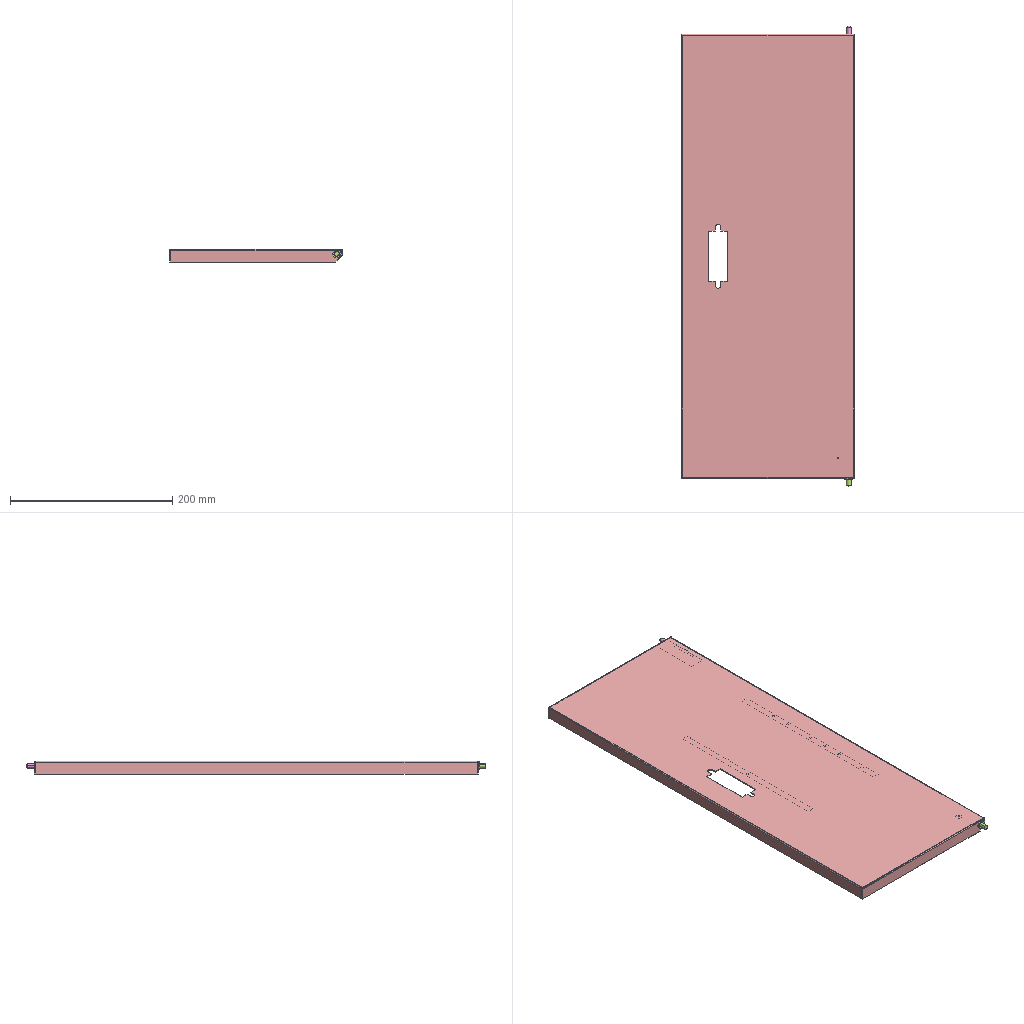Assembly | SolidWorks | 8 different items | 8 placed | box 213 x 566 x 17 mm
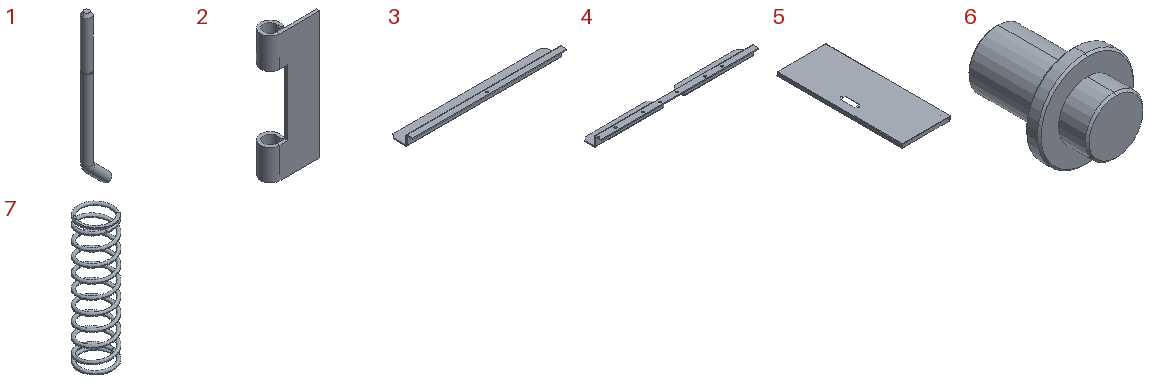Parts list (item | name | quantity | size | volume | features):
1 | - | x1 | 16.636 x 5.506 x 95.612 mm | 2325 mm3 | features Chamfer 2, ICE 2, Sweep 1
2 | - | x1 | 24 x 9.5 x 62 mm | 2570 mm3 | features FlatPattern 1, ICE 1, SMBaseFlange 1, SheetMetal 1
3 | - | x1 | 220 x 33.5 x 15 mm | 15208 mm3 | features EdgeFlange 2, ICE 2, Chamfer 1, FlatPattern 1, SMBaseFlange 1, SheetMetal 1
4 | - | x1 | 230 x 28.5 x 15 mm | 12722 mm3 | features LPattern 4, ICE 3, EdgeFlange 2, Chamfer 1, FlatPattern 1, SMBaseFlange 1, SheetMetal 1
5 | - | x1 | 213 x 547 x 16 mm | 163711 mm3 | features EdgeFlange 4, FlatPattern 1, ICE 1, SMBaseFlange 1, SheetMetal 1
6 | - | x1 | 10 x 12.5 x 10 mm | 426.85 mm3 | features ICE 2, Chamfer 1, Extrusion 1
7 | - | x1 | 8.799 x 8.797 x 32 mm | 125.702 mm3 | features BaseBody 1
8 | headless studs for stud welding gb | x1 | - | - | -
Mates (type | each side: item.copy, entity, surface, feature):
Coincident | 5.1 face plane Base-Flange1 | 2.1 face plane Base-Flange1
Coincident | 5.1 face plane Edge-Flange1 | 2.1 face plane Base-Bend1
DistanceDim | 2.1 face plane Base-Flange1 | 5.1 face plane Edge-Flange3
Concentric | 5.1 face cylinder Cut-Extrude1 | 6.1 face cylinder Boss-Extrude3
DistanceDim | 1.1 face plane Boss-Extrude2 | 5.1 face plane Edge-Flange1
Concentric | 2.1 face cylinder Base-Bend1 | 1.1 face cylinder Boss-Extrude2
Coincident | 2.1 face plane Cut-Extrude1 | 7.1 face plane Input1
Tangent | 2.1 face cylinder Base-Bend1 | 7.1 face surface:4006 Input1
Coincident | 5.1 face plane Edge-Flange1 | 6.1 face plane Boss-Extrude1
Coincident | 5.1 face plane Base-Flange1 | 3.1 face plane Edge-Flange2
Width | 5.1 face plane Edge-Flange1 | 5.1 face plane Edge-Flange1 | 3.1 face plane Base-Flange1 | 3.1 face plane Edge-Flange2
Coincident | 5.1 face plane Base-Flange1 | 4.1 face plane Edge-Flange2
Width | 5.1 face plane Edge-Flange1 | 5.1 face plane Edge-Flange1 | 4.1 face plane Base-Flange1 | 4.1 face plane Base-Flange1